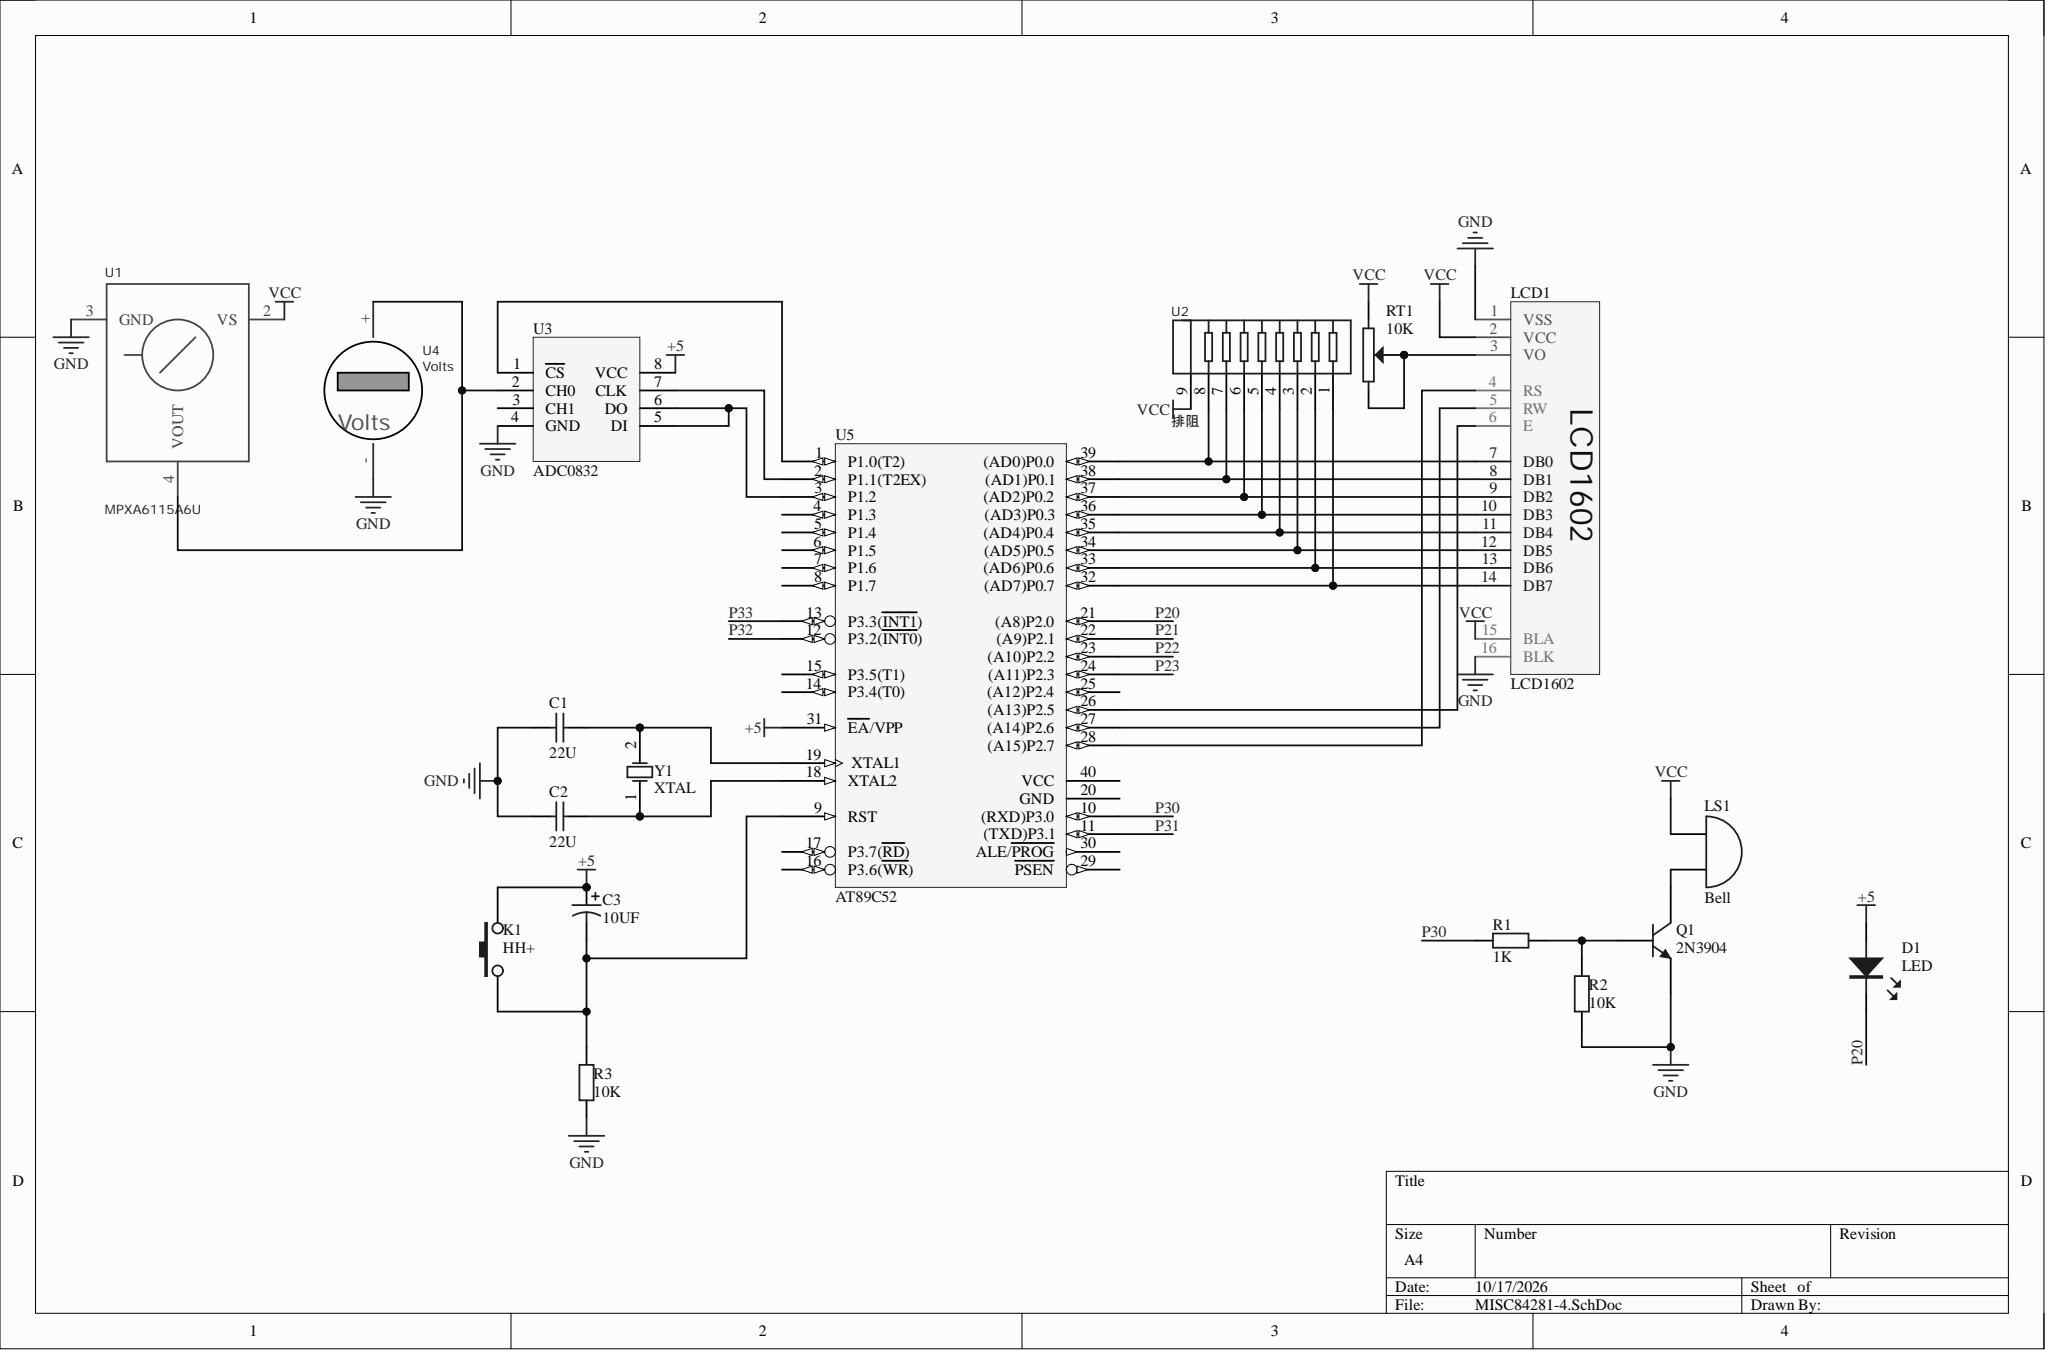Circuit board | Altium Designer | 18 parts | 26 nets
Bill of materials:
Comment,Description,Designator,Footprint,LibRef,Quantity
"22U","Capacitor","C1, C2","RAD-0.3","Cap","2"
"10UF","Polarized Capacitor (Radial)","C3","RB7.6-15","Cap Pol1","1"
"LED","","D1","LED5-BLUE","LED","1"
"HH+","","K1","四脚轻触开关","四脚轻触开关","1"
"LCD1602","","LCD1","LCD1602","LCD1602","1"
"Bell","Electrical Bell","LS1","PIN2","Bell","1"
"2N3904","NPN General Purpose Amplifier","Q1","TO-92A","2N3904","1"
"1K","Resistor","R1","AXIAL-0.4","Res2","1"
"10K","Resistor","R2, R3","AXIAL-0.4","Res2","2"
"10K","","RT1","电位器","电位器","1"
"MPXA6115A6U","","U1","482","MPXA6115A6U","1"
"排阻","","U2","paizu","排阻","1"
"ADC0832","U?","U3","P008","ADC0832","1"
"Volts","","U4","CAPACITANCE 1 FARAD 5,5 VOLT","Volts","1"
"AT89C52","","U5","DIP40","STC89C52","1"
"XTAL","Crystal Oscillator","Y1","R38","XTAL","1"
Netlist (Protel format):
[
C1
RAD-0.3
22U



]
[
C2
RAD-0.3
22U



]
[
C3
RB7.6-15
10UF



]
[
D1
LED5-BLUE
LED



]
[
K1
四脚轻触开关
HH+



]
[
LCD1
LCD1602
LCD1602



]
[
LS1
PIN2
Bell



]
[
Q1
TO-92A
2N3904



]
[
R1
AXIAL-0.4
1K



]
[
R2
AXIAL-0.4
10K



]
[
R3
AXIAL-0.4
10K



]
[
RT1
电位器
10K



]
[
U1
482
MPXA6115A6U



]
[
U2
paizu
排阻



]
[
U3
P008
ADC0832



]
[
U4
CAPACITANCE 1 FARAD 5,5 VOLT
Volts



]
[
U5
DIP40
AT89C52



]
[
Y1
R38
XTAL



]
(
VCC
LCD1-2
LCD1-15
LS1-1
RT1-1
U1-2
U2-9
)
(
P30
R1-2
U5-10
)
(
P20
D1-K
U5-21
)
(
NetU3_7
U3-7
U5-2
)
(
NetU3_5
U3-5
U3-6
U5-3
)
(
NetU3_1
U3-1
U5-1
)
(
NetU1_4
U1-4
U3-2
U4-+
)
(
NetQ1_2
Q1-2
R1-1
R2-2
)
(
NetLS1_2
LS1-2
Q1-3
)
(
NetLCD1_14
LCD1-14
U2-1
U5-32
)
(
NetLCD1_13
LCD1-13
U2-2
U5-33
)
(
NetLCD1_12
LCD1-12
U2-3
U5-34
)
(
NetLCD1_11
LCD1-11
U2-4
U5-35
)
(
NetLCD1_10
LCD1-10
U2-5
U5-36
)
(
NetLCD1_9
LCD1-9
U2-6
U5-37
)
(
NetLCD1_8
LCD1-8
U2-7
U5-38
)
(
NetLCD1_7
LCD1-7
U2-8
U5-39
)
(
NetLCD1_6
LCD1-6
U5-26
)
(
NetLCD1_5
LCD1-5
U5-27
)
(
NetLCD1_4
LCD1-4
U5-28
)
(
NetLCD1_3
LCD1-3
RT1-2
RT1-3
)
(
NetC3_2
C3-2
K1-1
R3-2
U5-9
)
(
NetC2_2
C2-2
U5-18
Y1-1
)
(
NetC1_2
C1-2
U5-19
Y1-2
)
(
GND
C1-1
C2-1
LCD1-1
LCD1-16
Q1-1
R2-1
R3-1
U1-3
U3-4
U4--
)
(
+5
C3-1
D1-A
K1-2
U3-8
U5-31
)